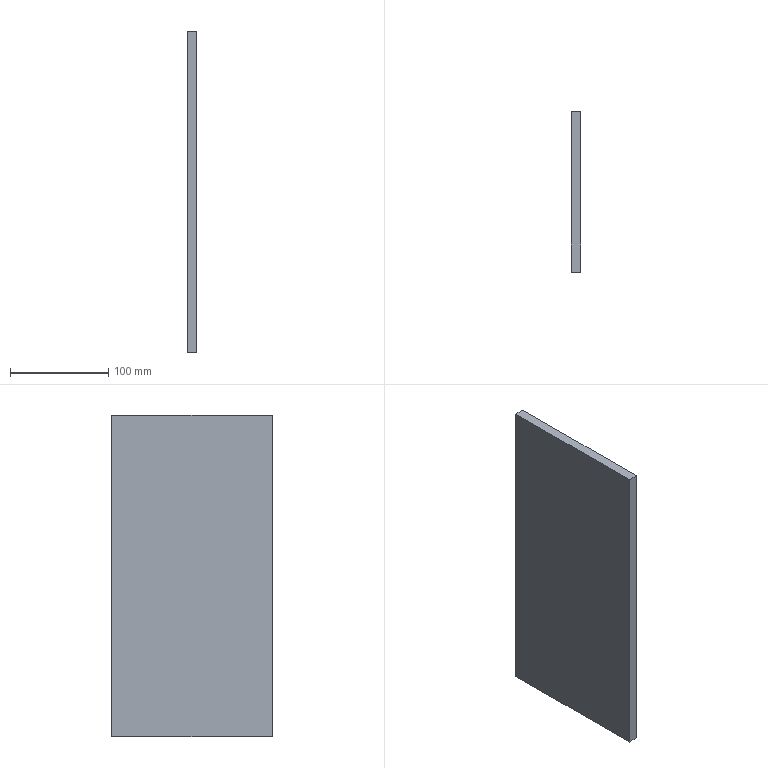Part | STEP file | 1 solid | 6 faces | box 10 x 164 x 327.57 mm | volume 537214 mm3 | plane 6
STEP:
#1=CARTESIAN_POINT('',(0.,0.,0.));
#2=DIRECTION('',(0.,0.,1.));
#3=DIRECTION('',(1.,0.,0.));
#4=AXIS2_PLACEMENT_3D('',#1,#2,#3);
#5=CARTESIAN_POINT('',(-81.848,-160.836,363.641));
#6=VERTEX_POINT('',#5);
#7=CARTESIAN_POINT('',(-81.848,3.164,363.641));
#8=VERTEX_POINT('',#7);
#9=CARTESIAN_POINT('',(-81.848,3.164,363.641));
#10=DIRECTION('',(0.,1.,0.));
#11=VECTOR('',#10,1.);
#12=LINE('',#9,#11);
#13=CARTESIAN_POINT('',(-71.848,3.164,363.641));
#14=DIRECTION('',(0.,0.,1.));
#15=DIRECTION('',(1.,0.,0.));
#16=AXIS2_PLACEMENT_3D('',#13,#14,#15);
#17=PLANE('',#16);
#18=CARTESIAN_POINT('',(-10.,0.));
#19=DIRECTION('',(0.,1.));
#20=VECTOR('',#19,1.);
#21=LINE('',#18,#20);
#22=(GEOMETRIC_REPRESENTATION_CONTEXT(2)PARAMETRIC_REPRESENTATION_CONTEXT()REPRESENTATION_CONTEXT('',''));
#23=DEFINITIONAL_REPRESENTATION('',(#21),#22);
#24=PCURVE('',#17,#23);
#25=CARTESIAN_POINT('',(-81.848,0.,0.));
#26=DIRECTION('',(1.,0.,0.));
#27=DIRECTION('',(0.,1.,0.));
#28=AXIS2_PLACEMENT_3D('',#25,#26,#27);
#29=PLANE('',#28);
#30=CARTESIAN_POINT('',(3.164,363.641));
#31=DIRECTION('',(1.,0.));
#32=VECTOR('',#31,1.);
#33=LINE('',#30,#32);
#34=(GEOMETRIC_REPRESENTATION_CONTEXT(2)PARAMETRIC_REPRESENTATION_CONTEXT()REPRESENTATION_CONTEXT('',''));
#35=DEFINITIONAL_REPRESENTATION('',(#33),#34);
#36=PCURVE('',#29,#35);
#37=SURFACE_CURVE('',#12,(#24,#36),.PCURVE_S1.);
#38=EDGE_CURVE('',#6,#8,#37,.T.);
#39=ORIENTED_EDGE('',*,*,#38,.F.);
#40=CARTESIAN_POINT('',(-71.848,-160.836,363.641));
#41=VERTEX_POINT('',#40);
#42=CARTESIAN_POINT('',(-71.848,-160.836,363.641));
#43=DIRECTION('',(-1.,0.,0.));
#44=VECTOR('',#43,1.);
#45=LINE('',#42,#44);
#46=CARTESIAN_POINT('',(0.,-164.));
#47=DIRECTION('',(-1.,0.));
#48=VECTOR('',#47,1.);
#49=LINE('',#46,#48);
#50=(GEOMETRIC_REPRESENTATION_CONTEXT(2)PARAMETRIC_REPRESENTATION_CONTEXT()REPRESENTATION_CONTEXT('',''));
#51=DEFINITIONAL_REPRESENTATION('',(#49),#50);
#52=PCURVE('',#17,#51);
#53=CARTESIAN_POINT('',(-71.848,-160.836,363.641));
#54=DIRECTION('',(0.,-1.,0.));
#55=DIRECTION('',(1.,0.,0.));
#56=AXIS2_PLACEMENT_3D('',#53,#54,#55);
#57=PLANE('',#56);
#58=CARTESIAN_POINT('',(0.,0.));
#59=DIRECTION('',(-1.,0.));
#60=VECTOR('',#59,1.);
#61=LINE('',#58,#60);
#62=(GEOMETRIC_REPRESENTATION_CONTEXT(2)PARAMETRIC_REPRESENTATION_CONTEXT()REPRESENTATION_CONTEXT('',''));
#63=DEFINITIONAL_REPRESENTATION('',(#61),#62);
#64=PCURVE('',#57,#63);
#65=SURFACE_CURVE('',#45,(#52,#64),.PCURVE_S1.);
#66=EDGE_CURVE('',#41,#6,#65,.T.);
#67=ORIENTED_EDGE('',*,*,#66,.F.);
#68=CARTESIAN_POINT('',(-71.848,3.164,363.641));
#69=VERTEX_POINT('',#68);
#70=CARTESIAN_POINT('',(-71.848,3.164,363.641));
#71=DIRECTION('',(0.,1.,0.));
#72=VECTOR('',#71,1.);
#73=LINE('',#70,#72);
#74=CARTESIAN_POINT('',(0.,0.));
#75=DIRECTION('',(0.,1.));
#76=VECTOR('',#75,1.);
#77=LINE('',#74,#76);
#78=(GEOMETRIC_REPRESENTATION_CONTEXT(2)PARAMETRIC_REPRESENTATION_CONTEXT()REPRESENTATION_CONTEXT('',''));
#79=DEFINITIONAL_REPRESENTATION('',(#77),#78);
#80=PCURVE('',#17,#79);
#81=CARTESIAN_POINT('',(-71.848,0.,0.));
#82=DIRECTION('',(1.,0.,0.));
#83=DIRECTION('',(0.,1.,0.));
#84=AXIS2_PLACEMENT_3D('',#81,#82,#83);
#85=PLANE('',#84);
#86=CARTESIAN_POINT('',(3.164,363.641));
#87=DIRECTION('',(1.,0.));
#88=VECTOR('',#87,1.);
#89=LINE('',#86,#88);
#90=(GEOMETRIC_REPRESENTATION_CONTEXT(2)PARAMETRIC_REPRESENTATION_CONTEXT()REPRESENTATION_CONTEXT('',''));
#91=DEFINITIONAL_REPRESENTATION('',(#89),#90);
#92=PCURVE('',#85,#91);
#93=SURFACE_CURVE('',#73,(#80,#92),.PCURVE_S1.);
#94=EDGE_CURVE('',#41,#69,#93,.T.);
#95=ORIENTED_EDGE('',*,*,#94,.T.);
#96=CARTESIAN_POINT('',(-71.848,3.164,363.641));
#97=DIRECTION('',(-1.,0.,0.));
#98=VECTOR('',#97,1.);
#99=LINE('',#96,#98);
#100=CARTESIAN_POINT('',(0.,0.));
#101=DIRECTION('',(-1.,0.));
#102=VECTOR('',#101,1.);
#103=LINE('',#100,#102);
#104=(GEOMETRIC_REPRESENTATION_CONTEXT(2)PARAMETRIC_REPRESENTATION_CONTEXT()REPRESENTATION_CONTEXT('',''));
#105=DEFINITIONAL_REPRESENTATION('',(#103),#104);
#106=PCURVE('',#17,#105);
#107=CARTESIAN_POINT('',(-71.848,3.164,363.641));
#108=DIRECTION('',(0.,1.,0.));
#109=DIRECTION('',(-1.,0.,0.));
#110=AXIS2_PLACEMENT_3D('',#107,#108,#109);
#111=PLANE('',#110);
#112=CARTESIAN_POINT('',(0.,0.));
#113=DIRECTION('',(1.,0.));
#114=VECTOR('',#113,1.);
#115=LINE('',#112,#114);
#116=(GEOMETRIC_REPRESENTATION_CONTEXT(2)PARAMETRIC_REPRESENTATION_CONTEXT()REPRESENTATION_CONTEXT('',''));
#117=DEFINITIONAL_REPRESENTATION('',(#115),#116);
#118=PCURVE('',#111,#117);
#119=SURFACE_CURVE('',#99,(#106,#118),.PCURVE_S1.);
#120=EDGE_CURVE('',#69,#8,#119,.T.);
#121=ORIENTED_EDGE('',*,*,#120,.T.);
#122=EDGE_LOOP('',(#39,#67,#95,#121));
#123=FACE_BOUND('',#122,.T.);
#124=ADVANCED_FACE('',(#123),#17,.T.);
#125=CARTESIAN_POINT('',(-81.848,-160.836,36.071));
#126=VERTEX_POINT('',#125);
#127=CARTESIAN_POINT('',(-81.848,-160.836,363.641));
#128=DIRECTION('',(0.,0.,1.));
#129=VECTOR('',#128,1.);
#130=LINE('',#127,#129);
#131=CARTESIAN_POINT('',(-10.,0.));
#132=DIRECTION('',(0.,1.));
#133=VECTOR('',#132,1.);
#134=LINE('',#131,#133);
#135=(GEOMETRIC_REPRESENTATION_CONTEXT(2)PARAMETRIC_REPRESENTATION_CONTEXT()REPRESENTATION_CONTEXT('',''));
#136=DEFINITIONAL_REPRESENTATION('',(#134),#135);
#137=PCURVE('',#57,#136);
#138=CARTESIAN_POINT('',(-160.836,363.641));
#139=DIRECTION('',(0.,1.));
#140=VECTOR('',#139,1.);
#141=LINE('',#138,#140);
#142=(GEOMETRIC_REPRESENTATION_CONTEXT(2)PARAMETRIC_REPRESENTATION_CONTEXT()REPRESENTATION_CONTEXT('',''));
#143=DEFINITIONAL_REPRESENTATION('',(#141),#142);
#144=PCURVE('',#29,#143);
#145=SURFACE_CURVE('',#130,(#137,#144),.PCURVE_S1.);
#146=EDGE_CURVE('',#126,#6,#145,.T.);
#147=ORIENTED_EDGE('',*,*,#146,.F.);
#148=CARTESIAN_POINT('',(-71.848,-160.836,36.071));
#149=VERTEX_POINT('',#148);
#150=CARTESIAN_POINT('',(-71.848,-160.836,36.071));
#151=DIRECTION('',(-1.,0.,0.));
#152=VECTOR('',#151,1.);
#153=LINE('',#150,#152);
#154=CARTESIAN_POINT('',(0.,-327.57));
#155=DIRECTION('',(-1.,0.));
#156=VECTOR('',#155,1.);
#157=LINE('',#154,#156);
#158=(GEOMETRIC_REPRESENTATION_CONTEXT(2)PARAMETRIC_REPRESENTATION_CONTEXT()REPRESENTATION_CONTEXT('',''));
#159=DEFINITIONAL_REPRESENTATION('',(#157),#158);
#160=PCURVE('',#57,#159);
#161=CARTESIAN_POINT('',(-71.848,3.164,36.071));
#162=DIRECTION('',(0.,0.,-1.));
#163=DIRECTION('',(-1.,0.,0.));
#164=AXIS2_PLACEMENT_3D('',#161,#162,#163);
#165=PLANE('',#164);
#166=CARTESIAN_POINT('',(0.,-164.));
#167=DIRECTION('',(1.,0.));
#168=VECTOR('',#167,1.);
#169=LINE('',#166,#168);
#170=(GEOMETRIC_REPRESENTATION_CONTEXT(2)PARAMETRIC_REPRESENTATION_CONTEXT()REPRESENTATION_CONTEXT('',''));
#171=DEFINITIONAL_REPRESENTATION('',(#169),#170);
#172=PCURVE('',#165,#171);
#173=SURFACE_CURVE('',#153,(#160,#172),.PCURVE_S1.);
#174=EDGE_CURVE('',#149,#126,#173,.T.);
#175=ORIENTED_EDGE('',*,*,#174,.F.);
#176=CARTESIAN_POINT('',(-71.848,-160.836,363.641));
#177=DIRECTION('',(0.,0.,1.));
#178=VECTOR('',#177,1.);
#179=LINE('',#176,#178);
#180=CARTESIAN_POINT('',(0.,0.));
#181=DIRECTION('',(0.,1.));
#182=VECTOR('',#181,1.);
#183=LINE('',#180,#182);
#184=(GEOMETRIC_REPRESENTATION_CONTEXT(2)PARAMETRIC_REPRESENTATION_CONTEXT()REPRESENTATION_CONTEXT('',''));
#185=DEFINITIONAL_REPRESENTATION('',(#183),#184);
#186=PCURVE('',#57,#185);
#187=CARTESIAN_POINT('',(-160.836,363.641));
#188=DIRECTION('',(0.,1.));
#189=VECTOR('',#188,1.);
#190=LINE('',#187,#189);
#191=(GEOMETRIC_REPRESENTATION_CONTEXT(2)PARAMETRIC_REPRESENTATION_CONTEXT()REPRESENTATION_CONTEXT('',''));
#192=DEFINITIONAL_REPRESENTATION('',(#190),#191);
#193=PCURVE('',#85,#192);
#194=SURFACE_CURVE('',#179,(#186,#193),.PCURVE_S1.);
#195=EDGE_CURVE('',#149,#41,#194,.T.);
#196=ORIENTED_EDGE('',*,*,#195,.T.);
#197=ORIENTED_EDGE('',*,*,#66,.T.);
#198=EDGE_LOOP('',(#147,#175,#196,#197));
#199=FACE_BOUND('',#198,.T.);
#200=ADVANCED_FACE('',(#199),#57,.T.);
#201=CARTESIAN_POINT('',(-81.848,3.164,36.071));
#202=VERTEX_POINT('',#201);
#203=CARTESIAN_POINT('',(-81.848,3.164,36.071));
#204=DIRECTION('',(0.,-1.,0.));
#205=VECTOR('',#204,1.);
#206=LINE('',#203,#205);
#207=CARTESIAN_POINT('',(10.,0.));
#208=DIRECTION('',(0.,-1.));
#209=VECTOR('',#208,1.);
#210=LINE('',#207,#209);
#211=(GEOMETRIC_REPRESENTATION_CONTEXT(2)PARAMETRIC_REPRESENTATION_CONTEXT()REPRESENTATION_CONTEXT('',''));
#212=DEFINITIONAL_REPRESENTATION('',(#210),#211);
#213=PCURVE('',#165,#212);
#214=CARTESIAN_POINT('',(3.164,36.071));
#215=DIRECTION('',(-1.,0.));
#216=VECTOR('',#215,1.);
#217=LINE('',#214,#216);
#218=(GEOMETRIC_REPRESENTATION_CONTEXT(2)PARAMETRIC_REPRESENTATION_CONTEXT()REPRESENTATION_CONTEXT('',''));
#219=DEFINITIONAL_REPRESENTATION('',(#217),#218);
#220=PCURVE('',#29,#219);
#221=SURFACE_CURVE('',#206,(#213,#220),.PCURVE_S1.);
#222=EDGE_CURVE('',#202,#126,#221,.T.);
#223=ORIENTED_EDGE('',*,*,#222,.F.);
#224=CARTESIAN_POINT('',(-71.848,3.164,36.071));
#225=VERTEX_POINT('',#224);
#226=CARTESIAN_POINT('',(-71.848,3.164,36.071));
#227=DIRECTION('',(-1.,0.,0.));
#228=VECTOR('',#227,1.);
#229=LINE('',#226,#228);
#230=CARTESIAN_POINT('',(0.,0.));
#231=DIRECTION('',(1.,0.));
#232=VECTOR('',#231,1.);
#233=LINE('',#230,#232);
#234=(GEOMETRIC_REPRESENTATION_CONTEXT(2)PARAMETRIC_REPRESENTATION_CONTEXT()REPRESENTATION_CONTEXT('',''));
#235=DEFINITIONAL_REPRESENTATION('',(#233),#234);
#236=PCURVE('',#165,#235);
#237=CARTESIAN_POINT('',(0.,-327.57));
#238=DIRECTION('',(1.,0.));
#239=VECTOR('',#238,1.);
#240=LINE('',#237,#239);
#241=(GEOMETRIC_REPRESENTATION_CONTEXT(2)PARAMETRIC_REPRESENTATION_CONTEXT()REPRESENTATION_CONTEXT('',''));
#242=DEFINITIONAL_REPRESENTATION('',(#240),#241);
#243=PCURVE('',#111,#242);
#244=SURFACE_CURVE('',#229,(#236,#243),.PCURVE_S1.);
#245=EDGE_CURVE('',#225,#202,#244,.T.);
#246=ORIENTED_EDGE('',*,*,#245,.F.);
#247=CARTESIAN_POINT('',(-71.848,3.164,36.071));
#248=DIRECTION('',(0.,-1.,0.));
#249=VECTOR('',#248,1.);
#250=LINE('',#247,#249);
#251=CARTESIAN_POINT('',(0.,0.));
#252=DIRECTION('',(0.,-1.));
#253=VECTOR('',#252,1.);
#254=LINE('',#251,#253);
#255=(GEOMETRIC_REPRESENTATION_CONTEXT(2)PARAMETRIC_REPRESENTATION_CONTEXT()REPRESENTATION_CONTEXT('',''));
#256=DEFINITIONAL_REPRESENTATION('',(#254),#255);
#257=PCURVE('',#165,#256);
#258=CARTESIAN_POINT('',(3.164,36.071));
#259=DIRECTION('',(-1.,0.));
#260=VECTOR('',#259,1.);
#261=LINE('',#258,#260);
#262=(GEOMETRIC_REPRESENTATION_CONTEXT(2)PARAMETRIC_REPRESENTATION_CONTEXT()REPRESENTATION_CONTEXT('',''));
#263=DEFINITIONAL_REPRESENTATION('',(#261),#262);
#264=PCURVE('',#85,#263);
#265=SURFACE_CURVE('',#250,(#257,#264),.PCURVE_S1.);
#266=EDGE_CURVE('',#225,#149,#265,.T.);
#267=ORIENTED_EDGE('',*,*,#266,.T.);
#268=ORIENTED_EDGE('',*,*,#174,.T.);
#269=EDGE_LOOP('',(#223,#246,#267,#268));
#270=FACE_BOUND('',#269,.T.);
#271=ADVANCED_FACE('',(#270),#165,.T.);
#272=CARTESIAN_POINT('',(-81.848,3.164,363.641));
#273=DIRECTION('',(0.,0.,-1.));
#274=VECTOR('',#273,1.);
#275=LINE('',#272,#274);
#276=CARTESIAN_POINT('',(10.,0.));
#277=DIRECTION('',(0.,-1.));
#278=VECTOR('',#277,1.);
#279=LINE('',#276,#278);
#280=(GEOMETRIC_REPRESENTATION_CONTEXT(2)PARAMETRIC_REPRESENTATION_CONTEXT()REPRESENTATION_CONTEXT('',''));
#281=DEFINITIONAL_REPRESENTATION('',(#279),#280);
#282=PCURVE('',#111,#281);
#283=CARTESIAN_POINT('',(3.164,363.641));
#284=DIRECTION('',(0.,-1.));
#285=VECTOR('',#284,1.);
#286=LINE('',#283,#285);
#287=(GEOMETRIC_REPRESENTATION_CONTEXT(2)PARAMETRIC_REPRESENTATION_CONTEXT()REPRESENTATION_CONTEXT('',''));
#288=DEFINITIONAL_REPRESENTATION('',(#286),#287);
#289=PCURVE('',#29,#288);
#290=SURFACE_CURVE('',#275,(#282,#289),.PCURVE_S1.);
#291=EDGE_CURVE('',#8,#202,#290,.T.);
#292=ORIENTED_EDGE('',*,*,#291,.F.);
#293=ORIENTED_EDGE('',*,*,#120,.F.);
#294=CARTESIAN_POINT('',(-71.848,3.164,363.641));
#295=DIRECTION('',(0.,0.,-1.));
#296=VECTOR('',#295,1.);
#297=LINE('',#294,#296);
#298=CARTESIAN_POINT('',(0.,0.));
#299=DIRECTION('',(0.,-1.));
#300=VECTOR('',#299,1.);
#301=LINE('',#298,#300);
#302=(GEOMETRIC_REPRESENTATION_CONTEXT(2)PARAMETRIC_REPRESENTATION_CONTEXT()REPRESENTATION_CONTEXT('',''));
#303=DEFINITIONAL_REPRESENTATION('',(#301),#302);
#304=PCURVE('',#111,#303);
#305=CARTESIAN_POINT('',(3.164,363.641));
#306=DIRECTION('',(0.,-1.));
#307=VECTOR('',#306,1.);
#308=LINE('',#305,#307);
#309=(GEOMETRIC_REPRESENTATION_CONTEXT(2)PARAMETRIC_REPRESENTATION_CONTEXT()REPRESENTATION_CONTEXT('',''));
#310=DEFINITIONAL_REPRESENTATION('',(#308),#309);
#311=PCURVE('',#85,#310);
#312=SURFACE_CURVE('',#297,(#304,#311),.PCURVE_S1.);
#313=EDGE_CURVE('',#69,#225,#312,.T.);
#314=ORIENTED_EDGE('',*,*,#313,.T.);
#315=ORIENTED_EDGE('',*,*,#245,.T.);
#316=EDGE_LOOP('',(#292,#293,#314,#315));
#317=FACE_BOUND('',#316,.T.);
#318=ADVANCED_FACE('',(#317),#111,.T.);
#319=ORIENTED_EDGE('',*,*,#94,.F.);
#320=ORIENTED_EDGE('',*,*,#195,.F.);
#321=ORIENTED_EDGE('',*,*,#266,.F.);
#322=ORIENTED_EDGE('',*,*,#313,.F.);
#323=EDGE_LOOP('',(#319,#320,#321,#322));
#324=FACE_BOUND('',#323,.T.);
#325=ADVANCED_FACE('',(#324),#85,.T.);
#326=ORIENTED_EDGE('',*,*,#38,.T.);
#327=ORIENTED_EDGE('',*,*,#291,.T.);
#328=ORIENTED_EDGE('',*,*,#222,.T.);
#329=ORIENTED_EDGE('',*,*,#146,.T.);
#330=EDGE_LOOP('',(#326,#327,#328,#329));
#331=FACE_BOUND('',#330,.T.);
#332=ADVANCED_FACE('',(#331),#29,.F.);
#333=CLOSED_SHELL('',(#124,#200,#271,#318,#325,#332));
#334=MANIFOLD_SOLID_BREP('',#333);
#335=(LENGTH_UNIT()NAMED_UNIT(*)SI_UNIT(.MILLI.,.METRE.));
#336=UNCERTAINTY_MEASURE_WITH_UNIT(LENGTH_MEASURE(0.0000001),#335,'','');
#337=(NAMED_UNIT(*)PLANE_ANGLE_UNIT()SI_UNIT($,.RADIAN.));
#338=(NAMED_UNIT(*)SI_UNIT($,.STERADIAN.)SOLID_ANGLE_UNIT());
#339=(GEOMETRIC_REPRESENTATION_CONTEXT(3)GLOBAL_UNCERTAINTY_ASSIGNED_CONTEXT((#336))GLOBAL_UNIT_ASSIGNED_CONTEXT((#335,#337,#338))REPRESENTATION_CONTEXT('',''));
#340=ADVANCED_BREP_SHAPE_REPRESENTATION('',(#4,#334),#339);